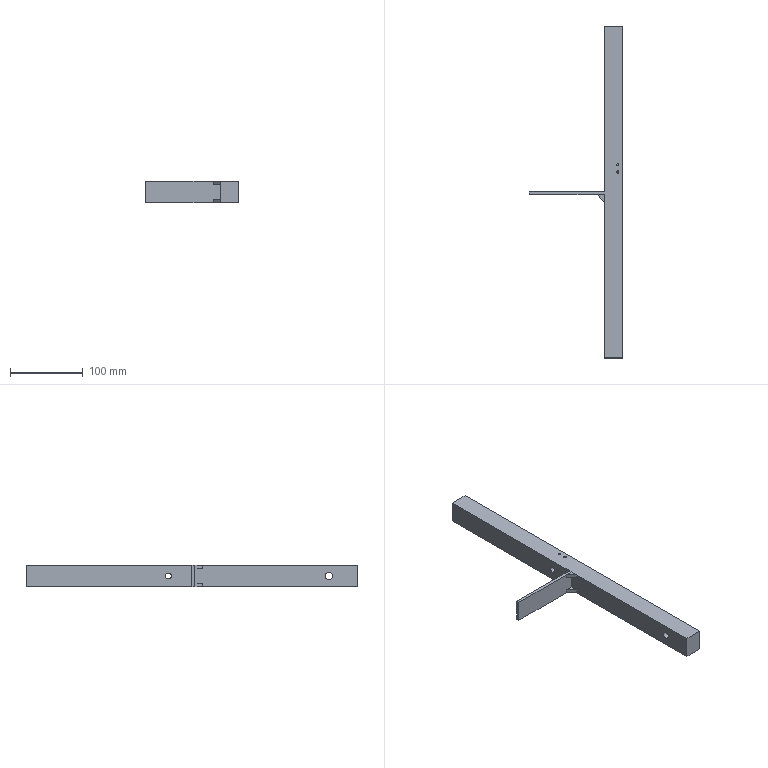Part | SolidWorks | features ICE 3, Cut 2, Gusset 2, Extrusion 1, Fillet 1, WeldmentFeature 1 | 3 solids | 37 faces | box 127.6 x 455 x 30 mm | volume 350644 mm3 | plane 24 | cylinder 13 | commonest cylinder face diameters 2 x5 3 x4 8 x2 10 x2
STEP:
#1=CARTESIAN_POINT('',(17.1,201.033,5.));
#2=VERTEX_POINT('',#1);
#3=CARTESIAN_POINT('',(20.1,201.033,5.));
#4=VERTEX_POINT('',#3);
#5=CARTESIAN_POINT('',(18.6,201.033,5.));
#6=DIRECTION('',(0.,0.,1.));
#7=DIRECTION('',(1.,0.,0.));
#8=AXIS2_PLACEMENT_3D('',#5,#6,#7);
#9=CIRCLE('',#8,1.5);
#10=EDGE_CURVE('',#2,#4,#9,.T.);
#11=ORIENTED_EDGE('',*,*,#10,.F.);
#12=CARTESIAN_POINT('',(17.1,201.033,15.));
#13=VERTEX_POINT('',#12);
#14=CARTESIAN_POINT('',(17.1,201.033,5.));
#15=DIRECTION('',(0.,0.,1.));
#16=VECTOR('',#15,1000.);
#17=LINE('',#14,#16);
#18=EDGE_CURVE('',#2,#13,#17,.T.);
#19=ORIENTED_EDGE('',*,*,#18,.T.);
#20=CARTESIAN_POINT('',(20.1,201.033,15.));
#21=VERTEX_POINT('',#20);
#22=CARTESIAN_POINT('',(18.6,201.033,15.));
#23=DIRECTION('',(0.,0.,1.));
#24=DIRECTION('',(1.,0.,0.));
#25=AXIS2_PLACEMENT_3D('',#22,#23,#24);
#26=CIRCLE('',#25,1.5);
#27=EDGE_CURVE('',#13,#21,#26,.T.);
#28=ORIENTED_EDGE('',*,*,#27,.T.);
#29=CARTESIAN_POINT('',(20.1,201.033,5.));
#30=DIRECTION('',(0.,0.,1.));
#31=VECTOR('',#30,1000.);
#32=LINE('',#29,#31);
#33=EDGE_CURVE('',#4,#21,#32,.T.);
#34=ORIENTED_EDGE('',*,*,#33,.F.);
#35=EDGE_LOOP('',(#11,#19,#28,#34));
#36=FACE_OUTER_BOUND('',#35,.T.);
#37=CARTESIAN_POINT('',(18.6,201.033,5.));
#38=DIRECTION('',(0.,0.,1.));
#39=DIRECTION('',(1.,0.,0.));
#40=AXIS2_PLACEMENT_3D('',#37,#38,#39);
#41=CYLINDRICAL_SURFACE('',#40,1.5);
#42=ADVANCED_FACE('',(#36),#41,.F.);
#43=CARTESIAN_POINT('',(17.1,211.033,5.));
#44=VERTEX_POINT('',#43);
#45=CARTESIAN_POINT('',(20.1,211.033,5.));
#46=VERTEX_POINT('',#45);
#47=CARTESIAN_POINT('',(18.6,211.033,5.));
#48=DIRECTION('',(0.,0.,1.));
#49=DIRECTION('',(1.,0.,0.));
#50=AXIS2_PLACEMENT_3D('',#47,#48,#49);
#51=CIRCLE('',#50,1.5);
#52=EDGE_CURVE('',#44,#46,#51,.T.);
#53=ORIENTED_EDGE('',*,*,#52,.F.);
#54=CARTESIAN_POINT('',(17.1,211.033,15.));
#55=VERTEX_POINT('',#54);
#56=CARTESIAN_POINT('',(17.1,211.033,5.));
#57=DIRECTION('',(0.,0.,1.));
#58=VECTOR('',#57,1000.);
#59=LINE('',#56,#58);
#60=EDGE_CURVE('',#44,#55,#59,.T.);
#61=ORIENTED_EDGE('',*,*,#60,.T.);
#62=CARTESIAN_POINT('',(20.1,211.033,15.));
#63=VERTEX_POINT('',#62);
#64=CARTESIAN_POINT('',(18.6,211.033,15.));
#65=DIRECTION('',(0.,0.,1.));
#66=DIRECTION('',(1.,0.,0.));
#67=AXIS2_PLACEMENT_3D('',#64,#65,#66);
#68=CIRCLE('',#67,1.5);
#69=EDGE_CURVE('',#55,#63,#68,.T.);
#70=ORIENTED_EDGE('',*,*,#69,.T.);
#71=CARTESIAN_POINT('',(20.1,211.033,5.));
#72=DIRECTION('',(0.,0.,1.));
#73=VECTOR('',#72,1000.);
#74=LINE('',#71,#73);
#75=EDGE_CURVE('',#46,#63,#74,.T.);
#76=ORIENTED_EDGE('',*,*,#75,.F.);
#77=EDGE_LOOP('',(#53,#61,#70,#76));
#78=FACE_OUTER_BOUND('',#77,.T.);
#79=CARTESIAN_POINT('',(18.6,211.033,5.));
#80=DIRECTION('',(0.,0.,1.));
#81=DIRECTION('',(1.,0.,0.));
#82=AXIS2_PLACEMENT_3D('',#79,#80,#81);
#83=CYLINDRICAL_SURFACE('',#82,1.5);
#84=ADVANCED_FACE('',(#78),#83,.F.);
#85=CARTESIAN_POINT('',(19.6,201.033,-5.));
#86=VERTEX_POINT('',#85);
#87=CARTESIAN_POINT('',(17.6,201.033,-5.));
#88=VERTEX_POINT('',#87);
#89=CARTESIAN_POINT('',(18.6,201.033,-5.));
#90=DIRECTION('',(0.,0.,-1.));
#91=DIRECTION('',(-1.,0.,0.));
#92=AXIS2_PLACEMENT_3D('',#89,#90,#91);
#93=CIRCLE('',#92,1.);
#94=EDGE_CURVE('',#86,#88,#93,.T.);
#95=ORIENTED_EDGE('',*,*,#94,.F.);
#96=CARTESIAN_POINT('',(19.6,201.033,-15.));
#97=VERTEX_POINT('',#96);
#98=CARTESIAN_POINT('',(19.6,201.033,-5.));
#99=DIRECTION('',(0.,0.,-1.));
#100=VECTOR('',#99,1000.);
#101=LINE('',#98,#100);
#102=EDGE_CURVE('',#86,#97,#101,.T.);
#103=ORIENTED_EDGE('',*,*,#102,.T.);
#104=CARTESIAN_POINT('',(17.6,201.033,-15.));
#105=VERTEX_POINT('',#104);
#106=CARTESIAN_POINT('',(18.6,201.033,-15.));
#107=DIRECTION('',(0.,0.,-1.));
#108=DIRECTION('',(-1.,0.,0.));
#109=AXIS2_PLACEMENT_3D('',#106,#107,#108);
#110=CIRCLE('',#109,1.);
#111=EDGE_CURVE('',#97,#105,#110,.T.);
#112=ORIENTED_EDGE('',*,*,#111,.T.);
#113=CARTESIAN_POINT('',(17.6,201.033,-5.));
#114=DIRECTION('',(0.,0.,-1.));
#115=VECTOR('',#114,1000.);
#116=LINE('',#113,#115);
#117=EDGE_CURVE('',#88,#105,#116,.T.);
#118=ORIENTED_EDGE('',*,*,#117,.F.);
#119=EDGE_LOOP('',(#95,#103,#112,#118));
#120=FACE_OUTER_BOUND('',#119,.T.);
#121=CARTESIAN_POINT('',(18.6,201.033,-5.));
#122=DIRECTION('',(0.,0.,-1.));
#123=DIRECTION('',(-1.,0.,0.));
#124=AXIS2_PLACEMENT_3D('',#121,#122,#123);
#125=CYLINDRICAL_SURFACE('',#124,1.);
#126=ADVANCED_FACE('',(#120),#125,.F.);
#127=CARTESIAN_POINT('',(19.6,211.033,-5.));
#128=VERTEX_POINT('',#127);
#129=CARTESIAN_POINT('',(17.6,211.033,-5.));
#130=VERTEX_POINT('',#129);
#131=CARTESIAN_POINT('',(18.6,211.033,-5.));
#132=DIRECTION('',(0.,0.,-1.));
#133=DIRECTION('',(-1.,0.,0.));
#134=AXIS2_PLACEMENT_3D('',#131,#132,#133);
#135=CIRCLE('',#134,1.);
#136=EDGE_CURVE('',#128,#130,#135,.T.);
#137=ORIENTED_EDGE('',*,*,#136,.F.);
#138=CARTESIAN_POINT('',(19.6,211.033,-15.));
#139=VERTEX_POINT('',#138);
#140=CARTESIAN_POINT('',(19.6,211.033,-5.));
#141=DIRECTION('',(0.,0.,-1.));
#142=VECTOR('',#141,1000.);
#143=LINE('',#140,#142);
#144=EDGE_CURVE('',#128,#139,#143,.T.);
#145=ORIENTED_EDGE('',*,*,#144,.T.);
#146=CARTESIAN_POINT('',(17.6,211.033,-15.));
#147=VERTEX_POINT('',#146);
#148=CARTESIAN_POINT('',(18.6,211.033,-15.));
#149=DIRECTION('',(0.,0.,-1.));
#150=DIRECTION('',(-1.,0.,0.));
#151=AXIS2_PLACEMENT_3D('',#148,#149,#150);
#152=CIRCLE('',#151,1.);
#153=EDGE_CURVE('',#139,#147,#152,.T.);
#154=ORIENTED_EDGE('',*,*,#153,.T.);
#155=CARTESIAN_POINT('',(17.6,211.033,-5.));
#156=DIRECTION('',(0.,0.,-1.));
#157=VECTOR('',#156,1000.);
#158=LINE('',#155,#157);
#159=EDGE_CURVE('',#130,#147,#158,.T.);
#160=ORIENTED_EDGE('',*,*,#159,.F.);
#161=EDGE_LOOP('',(#137,#145,#154,#160));
#162=FACE_OUTER_BOUND('',#161,.T.);
#163=CARTESIAN_POINT('',(18.6,211.033,-5.));
#164=DIRECTION('',(0.,0.,-1.));
#165=DIRECTION('',(-1.,0.,0.));
#166=AXIS2_PLACEMENT_3D('',#163,#164,#165);
#167=CYLINDRICAL_SURFACE('',#166,1.);
#168=ADVANCED_FACE('',(#162),#167,.F.);
#169=CARTESIAN_POINT('',(25.,-13.967,-5.));
#170=VERTEX_POINT('',#169);
#171=CARTESIAN_POINT('',(25.,-13.967,5.));
#172=VERTEX_POINT('',#171);
#173=CARTESIAN_POINT('',(25.,-13.967,0.));
#174=DIRECTION('',(-1.,0.,0.));
#175=DIRECTION('',(0.,-1.,0.));
#176=AXIS2_PLACEMENT_3D('',#173,#174,#175);
#177=CIRCLE('',#176,5.);
#178=EDGE_CURVE('',#170,#172,#177,.T.);
#179=ORIENTED_EDGE('',*,*,#178,.F.);
#180=CARTESIAN_POINT('',(0.,-13.967,-5.));
#181=VERTEX_POINT('',#180);
#182=CARTESIAN_POINT('',(66.,-13.967,-5.));
#183=DIRECTION('',(-1.,0.,0.));
#184=VECTOR('',#183,1000.);
#185=LINE('',#182,#184);
#186=EDGE_CURVE('',#170,#181,#185,.T.);
#187=ORIENTED_EDGE('',*,*,#186,.T.);
#188=CARTESIAN_POINT('',(0.,-13.967,5.));
#189=VERTEX_POINT('',#188);
#190=CARTESIAN_POINT('',(0.,-13.967,0.));
#191=DIRECTION('',(1.,0.,0.));
#192=DIRECTION('',(0.,0.,-1.));
#193=AXIS2_PLACEMENT_3D('',#190,#191,#192);
#194=CIRCLE('',#193,5.);
#195=EDGE_CURVE('',#189,#181,#194,.T.);
#196=ORIENTED_EDGE('',*,*,#195,.F.);
#197=CARTESIAN_POINT('',(66.,-13.967,5.));
#198=DIRECTION('',(-1.,0.,0.));
#199=VECTOR('',#198,1000.);
#200=LINE('',#197,#199);
#201=EDGE_CURVE('',#172,#189,#200,.T.);
#202=ORIENTED_EDGE('',*,*,#201,.F.);
#203=EDGE_LOOP('',(#179,#187,#196,#202));
#204=FACE_OUTER_BOUND('',#203,.T.);
#205=CARTESIAN_POINT('',(66.,-13.967,0.));
#206=DIRECTION('',(-1.,0.,0.));
#207=DIRECTION('',(0.,0.,1.));
#208=AXIS2_PLACEMENT_3D('',#205,#206,#207);
#209=CYLINDRICAL_SURFACE('',#208,5.);
#210=ADVANCED_FACE('',(#204),#209,.F.);
#211=CARTESIAN_POINT('',(25.,206.033,-4.));
#212=VERTEX_POINT('',#211);
#213=CARTESIAN_POINT('',(25.,206.033,4.));
#214=VERTEX_POINT('',#213);
#215=CARTESIAN_POINT('',(25.,206.033,0.));
#216=DIRECTION('',(-1.,0.,0.));
#217=DIRECTION('',(0.,-1.,0.));
#218=AXIS2_PLACEMENT_3D('',#215,#216,#217);
#219=CIRCLE('',#218,4.);
#220=EDGE_CURVE('',#212,#214,#219,.T.);
#221=ORIENTED_EDGE('',*,*,#220,.F.);
#222=CARTESIAN_POINT('',(0.,206.033,-4.));
#223=VERTEX_POINT('',#222);
#224=CARTESIAN_POINT('',(66.,206.033,-4.));
#225=DIRECTION('',(-1.,0.,0.));
#226=VECTOR('',#225,1000.);
#227=LINE('',#224,#226);
#228=EDGE_CURVE('',#212,#223,#227,.T.);
#229=ORIENTED_EDGE('',*,*,#228,.T.);
#230=CARTESIAN_POINT('',(0.,206.033,4.));
#231=VERTEX_POINT('',#230);
#232=CARTESIAN_POINT('',(0.,206.033,0.));
#233=DIRECTION('',(1.,0.,0.));
#234=DIRECTION('',(0.,0.,-1.));
#235=AXIS2_PLACEMENT_3D('',#232,#233,#234);
#236=CIRCLE('',#235,4.);
#237=EDGE_CURVE('',#231,#223,#236,.T.);
#238=ORIENTED_EDGE('',*,*,#237,.F.);
#239=CARTESIAN_POINT('',(66.,206.033,4.));
#240=DIRECTION('',(-1.,0.,0.));
#241=VECTOR('',#240,1000.);
#242=LINE('',#239,#241);
#243=EDGE_CURVE('',#214,#231,#242,.T.);
#244=ORIENTED_EDGE('',*,*,#243,.F.);
#245=EDGE_LOOP('',(#221,#229,#238,#244));
#246=FACE_OUTER_BOUND('',#245,.T.);
#247=CARTESIAN_POINT('',(66.,206.033,0.));
#248=DIRECTION('',(-1.,0.,0.));
#249=DIRECTION('',(0.,0.,1.));
#250=AXIS2_PLACEMENT_3D('',#247,#248,#249);
#251=CYLINDRICAL_SURFACE('',#250,4.);
#252=ADVANCED_FACE('',(#246),#251,.F.);
#253=ORIENTED_EDGE('',*,*,#237,.T.);
#254=CARTESIAN_POINT('',(0.,206.033,0.));
#255=DIRECTION('',(1.,0.,0.));
#256=DIRECTION('',(0.,0.,-1.));
#257=AXIS2_PLACEMENT_3D('',#254,#255,#256);
#258=CIRCLE('',#257,4.);
#259=EDGE_CURVE('',#223,#231,#258,.T.);
#260=ORIENTED_EDGE('',*,*,#259,.T.);
#261=EDGE_LOOP('',(#253,#260));
#262=FACE_BOUND('',#261,.T.);
#263=CARTESIAN_POINT('',(0.,401.033,-15.));
#264=VERTEX_POINT('',#263);
#265=CARTESIAN_POINT('',(0.,174.533,-15.));
#266=VERTEX_POINT('',#265);
#267=CARTESIAN_POINT('',(0.,0.,-15.));
#268=DIRECTION('',(0.,-1.,0.));
#269=VECTOR('',#268,1000.);
#270=LINE('',#267,#269);
#271=EDGE_CURVE('',#264,#266,#270,.T.);
#272=ORIENTED_EDGE('',*,*,#271,.T.);
#273=CARTESIAN_POINT('',(0.,174.533,15.));
#274=VERTEX_POINT('',#273);
#275=CARTESIAN_POINT('',(0.,174.533,15.));
#276=DIRECTION('',(0.,0.,1.));
#277=VECTOR('',#276,1000.);
#278=LINE('',#275,#277);
#279=EDGE_CURVE('',#266,#274,#278,.T.);
#280=ORIENTED_EDGE('',*,*,#279,.T.);
#281=CARTESIAN_POINT('',(0.,401.033,15.));
#282=VERTEX_POINT('',#281);
#283=CARTESIAN_POINT('',(0.,-53.967,15.));
#284=DIRECTION('',(0.,-1.,0.));
#285=VECTOR('',#284,1000.);
#286=LINE('',#283,#285);
#287=EDGE_CURVE('',#282,#274,#286,.T.);
#288=ORIENTED_EDGE('',*,*,#287,.F.);
#289=CARTESIAN_POINT('',(0.,401.033,-15.));
#290=DIRECTION('',(0.,0.,1.));
#291=VECTOR('',#290,1000.);
#292=LINE('',#289,#291);
#293=EDGE_CURVE('',#264,#282,#292,.T.);
#294=ORIENTED_EDGE('',*,*,#293,.F.);
#295=EDGE_LOOP('',(#272,#280,#288,#294));
#296=FACE_OUTER_BOUND('',#295,.T.);
#297=CARTESIAN_POINT('',(0.,0.,15.));
#298=DIRECTION('',(1.,0.,0.));
#299=DIRECTION('',(0.,0.,-1.));
#300=AXIS2_PLACEMENT_3D('',#297,#298,#299);
#301=PLANE('',#300);
#302=ADVANCED_FACE('',(#262,#296),#301,.F.);
#303=CARTESIAN_POINT('',(0.,-53.967,-15.));
#304=VERTEX_POINT('',#303);
#305=CARTESIAN_POINT('',(25.,-53.967,-15.));
#306=VERTEX_POINT('',#305);
#307=CARTESIAN_POINT('',(25.,-53.967,-15.));
#308=DIRECTION('',(1.,0.,0.));
#309=VECTOR('',#308,1000.);
#310=LINE('',#307,#309);
#311=EDGE_CURVE('',#304,#306,#310,.T.);
#312=ORIENTED_EDGE('',*,*,#311,.T.);
#313=CARTESIAN_POINT('',(25.,-53.967,15.));
#314=VERTEX_POINT('',#313);
#315=CARTESIAN_POINT('',(25.,-53.967,15.));
#316=DIRECTION('',(0.,0.,-1.));
#317=VECTOR('',#316,1000.);
#318=LINE('',#315,#317);
#319=EDGE_CURVE('',#314,#306,#318,.T.);
#320=ORIENTED_EDGE('',*,*,#319,.F.);
#321=CARTESIAN_POINT('',(0.,-53.967,15.));
#322=VERTEX_POINT('',#321);
#323=CARTESIAN_POINT('',(25.,-53.967,15.));
#324=DIRECTION('',(1.,0.,0.));
#325=VECTOR('',#324,1000.);
#326=LINE('',#323,#325);
#327=EDGE_CURVE('',#322,#314,#326,.T.);
#328=ORIENTED_EDGE('',*,*,#327,.F.);
#329=CARTESIAN_POINT('',(0.,-53.967,15.));
#330=DIRECTION('',(0.,0.,-1.));
#331=VECTOR('',#330,1000.);
#332=LINE('',#329,#331);
#333=EDGE_CURVE('',#322,#304,#332,.T.);
#334=ORIENTED_EDGE('',*,*,#333,.T.);
#335=EDGE_LOOP('',(#312,#320,#328,#334));
#336=FACE_OUTER_BOUND('',#335,.T.);
#337=CARTESIAN_POINT('',(25.,-53.967,15.));
#338=DIRECTION('',(0.,1.,0.));
#339=DIRECTION('',(-1.,0.,0.));
#340=AXIS2_PLACEMENT_3D('',#337,#338,#339);
#341=PLANE('',#340);
#342=ADVANCED_FACE('',(#336),#341,.F.);
#343=CARTESIAN_POINT('',(25.,-13.967,0.));
#344=DIRECTION('',(-1.,0.,0.));
#345=DIRECTION('',(0.,-1.,0.));
#346=AXIS2_PLACEMENT_3D('',#343,#344,#345);
#347=CIRCLE('',#346,5.);
#348=EDGE_CURVE('',#172,#170,#347,.T.);
#349=ORIENTED_EDGE('',*,*,#348,.T.);
#350=ORIENTED_EDGE('',*,*,#178,.T.);
#351=EDGE_LOOP('',(#349,#350));
#352=FACE_BOUND('',#351,.T.);
#353=CARTESIAN_POINT('',(25.,206.033,0.));
#354=DIRECTION('',(-1.,0.,0.));
#355=DIRECTION('',(0.,-1.,0.));
#356=AXIS2_PLACEMENT_3D('',#353,#354,#355);
#357=CIRCLE('',#356,4.);
#358=EDGE_CURVE('',#214,#212,#357,.T.);
#359=ORIENTED_EDGE('',*,*,#358,.T.);
#360=ORIENTED_EDGE('',*,*,#220,.T.);
#361=EDGE_LOOP('',(#359,#360));
#362=FACE_BOUND('',#361,.T.);
#363=CARTESIAN_POINT('',(25.,401.033,-15.));
#364=VERTEX_POINT('',#363);
#365=CARTESIAN_POINT('',(25.,246.033,-15.));
#366=DIRECTION('',(0.,1.,0.));
#367=VECTOR('',#366,1000.);
#368=LINE('',#365,#367);
#369=EDGE_CURVE('',#306,#364,#368,.T.);
#370=ORIENTED_EDGE('',*,*,#369,.T.);
#371=CARTESIAN_POINT('',(25.,401.033,15.));
#372=VERTEX_POINT('',#371);
#373=CARTESIAN_POINT('',(25.,401.033,15.));
#374=DIRECTION('',(0.,0.,-1.));
#375=VECTOR('',#374,1000.);
#376=LINE('',#373,#375);
#377=EDGE_CURVE('',#372,#364,#376,.T.);
#378=ORIENTED_EDGE('',*,*,#377,.F.);
#379=CARTESIAN_POINT('',(25.,-38.967,15.));
#380=DIRECTION('',(0.,1.,0.));
#381=VECTOR('',#380,1000.);
#382=LINE('',#379,#381);
#383=EDGE_CURVE('',#314,#372,#382,.T.);
#384=ORIENTED_EDGE('',*,*,#383,.F.);
#385=ORIENTED_EDGE('',*,*,#319,.T.);
#386=EDGE_LOOP('',(#370,#378,#384,#385));
#387=FACE_OUTER_BOUND('',#386,.T.);
#388=CARTESIAN_POINT('',(25.,246.033,15.));
#389=DIRECTION('',(-1.,0.,0.));
#390=DIRECTION('',(0.,-1.,0.));
#391=AXIS2_PLACEMENT_3D('',#388,#389,#390);
#392=PLANE('',#391);
#393=ADVANCED_FACE('',(#352,#362,#387),#392,.F.);
#394=ORIENTED_EDGE('',*,*,#195,.T.);
#395=CARTESIAN_POINT('',(0.,-13.967,0.));
#396=DIRECTION('',(1.,0.,0.));
#397=DIRECTION('',(0.,0.,-1.));
#398=AXIS2_PLACEMENT_3D('',#395,#396,#397);
#399=CIRCLE('',#398,5.);
#400=EDGE_CURVE('',#181,#189,#399,.T.);
#401=ORIENTED_EDGE('',*,*,#400,.T.);
#402=EDGE_LOOP('',(#394,#401));
#403=FACE_BOUND('',#402,.T.);
#404=CARTESIAN_POINT('',(0.,169.533,15.));
#405=VERTEX_POINT('',#404);
#406=CARTESIAN_POINT('',(0.,-53.967,15.));
#407=DIRECTION('',(0.,-1.,0.));
#408=VECTOR('',#407,1000.);
#409=LINE('',#406,#408);
#410=EDGE_CURVE('',#405,#322,#409,.T.);
#411=ORIENTED_EDGE('',*,*,#410,.F.);
#412=CARTESIAN_POINT('',(0.,169.533,-15.));
#413=VERTEX_POINT('',#412);
#414=CARTESIAN_POINT('',(0.,169.533,117.678));
#415=DIRECTION('',(0.,0.,-1.));
#416=VECTOR('',#415,1000.);
#417=LINE('',#414,#416);
#418=EDGE_CURVE('',#405,#413,#417,.T.);
#419=ORIENTED_EDGE('',*,*,#418,.T.);
#420=CARTESIAN_POINT('',(0.,0.,-15.));
#421=DIRECTION('',(0.,-1.,0.));
#422=VECTOR('',#421,1000.);
#423=LINE('',#420,#422);
#424=EDGE_CURVE('',#413,#304,#423,.T.);
#425=ORIENTED_EDGE('',*,*,#424,.T.);
#426=ORIENTED_EDGE('',*,*,#333,.F.);
#427=EDGE_LOOP('',(#411,#419,#425,#426));
#428=FACE_OUTER_BOUND('',#427,.T.);
#429=CARTESIAN_POINT('',(0.,0.,15.));
#430=DIRECTION('',(1.,0.,0.));
#431=DIRECTION('',(0.,0.,-1.));
#432=AXIS2_PLACEMENT_3D('',#429,#430,#431);
#433=PLANE('',#432);
#434=ADVANCED_FACE('',(#403,#428),#433,.F.);
#435=CARTESIAN_POINT('',(18.6,201.033,15.));
#436=DIRECTION('',(0.,0.,1.));
#437=DIRECTION('',(1.,0.,0.));
#438=AXIS2_PLACEMENT_3D('',#435,#436,#437);
#439=CIRCLE('',#438,1.5);
#440=EDGE_CURVE('',#21,#13,#439,.T.);
#441=ORIENTED_EDGE('',*,*,#440,.F.);
#442=ORIENTED_EDGE('',*,*,#27,.F.);
#443=EDGE_LOOP('',(#441,#442));
#444=FACE_BOUND('',#443,.T.);
#445=CARTESIAN_POINT('',(18.6,211.033,15.));
#446=DIRECTION('',(0.,0.,1.));
#447=DIRECTION('',(1.,0.,0.));
#448=AXIS2_PLACEMENT_3D('',#445,#446,#447);
#449=CIRCLE('',#448,1.5);
#450=EDGE_CURVE('',#63,#55,#449,.T.);
#451=ORIENTED_EDGE('',*,*,#450,.F.);
#452=ORIENTED_EDGE('',*,*,#69,.F.);
#453=EDGE_LOOP('',(#451,#452));
#454=FACE_BOUND('',#453,.T.);
#455=ORIENTED_EDGE('',*,*,#287,.T.);
#456=CARTESIAN_POINT('',(-1.,173.533,15.));
#457=VERTEX_POINT('',#456);
#458=CARTESIAN_POINT('',(-1.,174.533,15.));
#459=DIRECTION('',(0.,0.,-1.));
#460=DIRECTION('',(-1.,0.,0.));
#461=AXIS2_PLACEMENT_3D('',#458,#459,#460);
#462=CIRCLE('',#461,1.);
#463=EDGE_CURVE('',#274,#457,#462,.T.);
#464=ORIENTED_EDGE('',*,*,#463,.T.);
#465=CARTESIAN_POINT('',(-102.6,173.533,15.));
#466=VERTEX_POINT('',#465);
#467=CARTESIAN_POINT('',(0.,173.533,15.));
#468=DIRECTION('',(-1.,0.,0.));
#469=VECTOR('',#468,1000.);
#470=LINE('',#467,#469);
#471=EDGE_CURVE('',#457,#466,#470,.T.);
#472=ORIENTED_EDGE('',*,*,#471,.T.);
#473=CARTESIAN_POINT('',(-102.6,169.533,15.));
#474=VERTEX_POINT('',#473);
#475=CARTESIAN_POINT('',(-102.6,173.533,15.));
#476=DIRECTION('',(0.,-1.,0.));
#477=VECTOR('',#476,1000.);
#478=LINE('',#475,#477);
#479=EDGE_CURVE('',#466,#474,#478,.T.);
#480=ORIENTED_EDGE('',*,*,#479,.T.);
#481=CARTESIAN_POINT('',(-102.6,169.533,15.));
#482=DIRECTION('',(1.,0.,0.));
#483=VECTOR('',#482,1000.);
#484=LINE('',#481,#483);
#485=EDGE_CURVE('',#474,#405,#484,.T.);
#486=ORIENTED_EDGE('',*,*,#485,.T.);
#487=ORIENTED_EDGE('',*,*,#410,.T.);
#488=ORIENTED_EDGE('',*,*,#327,.T.);
#489=ORIENTED_EDGE('',*,*,#383,.T.);
#490=CARTESIAN_POINT('',(0.,401.033,15.));
#491=DIRECTION('',(1.,0.,0.));
#492=VECTOR('',#491,1000.);
#493=LINE('',#490,#492);
#494=EDGE_CURVE('',#282,#372,#493,.T.);
#495=ORIENTED_EDGE('',*,*,#494,.F.);
#496=EDGE_LOOP('',(#455,#464,#472,#480,#486,#487,#488,#489,#495));
#497=FACE_OUTER_BOUND('',#496,.T.);
#498=CARTESIAN_POINT('',(0.,0.,15.));
#499=DIRECTION('',(0.,0.,-1.));
#500=DIRECTION('',(-1.,0.,0.));
#501=AXIS2_PLACEMENT_3D('',#498,#499,#500);
#502=PLANE('',#501);
#503=ADVANCED_FACE('',(#444,#454,#497),#502,.F.);
#504=CARTESIAN_POINT('',(18.6,201.033,-15.));
#505=DIRECTION('',(0.,0.,-1.));
#506=DIRECTION('',(-1.,0.,0.));
#507=AXIS2_PLACEMENT_3D('',#504,#505,#506);
#508=CIRCLE('',#507,1.);
#509=EDGE_CURVE('',#105,#97,#508,.T.);
#510=ORIENTED_EDGE('',*,*,#509,.F.);
#511=ORIENTED_EDGE('',*,*,#111,.F.);
#512=EDGE_LOOP('',(#510,#511));
#513=FACE_BOUND('',#512,.T.);
#514=CARTESIAN_POINT('',(18.6,211.033,-15.));
#515=DIRECTION('',(0.,0.,-1.));
#516=DIRECTION('',(-1.,0.,0.));
#517=AXIS2_PLACEMENT_3D('',#514,#515,#516);
#518=CIRCLE('',#517,1.);
#519=EDGE_CURVE('',#147,#139,#518,.T.);
#520=ORIENTED_EDGE('',*,*,#519,.F.);
#521=ORIENTED_EDGE('',*,*,#153,.F.);
#522=EDGE_LOOP('',(#520,#521));
#523=FACE_BOUND('',#522,.T.);
#524=ORIENTED_EDGE('',*,*,#311,.F.);
#525=ORIENTED_EDGE('',*,*,#424,.F.);
#526=CARTESIAN_POINT('',(-102.6,169.533,-15.));
#527=VERTEX_POINT('',#526);
#528=CARTESIAN_POINT('',(-102.6,169.533,-15.));
#529=DIRECTION('',(-1.,0.,0.));
#530=VECTOR('',#529,1000.);
#531=LINE('',#528,#530);
#532=EDGE_CURVE('',#413,#527,#531,.T.);
#533=ORIENTED_EDGE('',*,*,#532,.T.);
#534=CARTESIAN_POINT('',(-102.6,173.533,-15.));
#535=VERTEX_POINT('',#534);
#536=CARTESIAN_POINT('',(-102.6,173.533,-15.));
#537=DIRECTION('',(0.,1.,0.));
#538=VECTOR('',#537,1000.);
#539=LINE('',#536,#538);
#540=EDGE_CURVE('',#527,#535,#539,.T.);
#541=ORIENTED_EDGE('',*,*,#540,.T.);
#542=CARTESIAN_POINT('',(-1.,173.533,-15.));
#543=VERTEX_POINT('',#542);
#544=CARTESIAN_POINT('',(0.,173.533,-15.));
#545=DIRECTION('',(1.,0.,0.));
#546=VECTOR('',#545,1000.);
#547=LINE('',#544,#546);
#548=EDGE_CURVE('',#535,#543,#547,.T.);
#549=ORIENTED_EDGE('',*,*,#548,.T.);
#550=CARTESIAN_POINT('',(-1.,174.533,-15.));
#551=DIRECTION('',(0.,0.,1.));
#552=DIRECTION('',(-1.,0.,0.));
#553=AXIS2_PLACEMENT_3D('',#550,#551,#552);
#554=CIRCLE('',#553,1.);
#555=EDGE_CURVE('',#543,#266,#554,.T.);
#556=ORIENTED_EDGE('',*,*,#555,.T.);
#557=ORIENTED_EDGE('',*,*,#271,.F.);
#558=CARTESIAN_POINT('',(25.,401.033,-15.));
#559=DIRECTION('',(-1.,0.,0.));
#560=VECTOR('',#559,1000.);
#561=LINE('',#558,#560);
#562=EDGE_CURVE('',#364,#264,#561,.T.);
#563=ORIENTED_EDGE('',*,*,#562,.F.);
#564=ORIENTED_EDGE('',*,*,#369,.F.);
#565=EDGE_LOOP('',(#524,#525,#533,#541,#549,#556,#557,#563,#564));
#566=FACE_OUTER_BOUND('',#565,.T.);
#567=CARTESIAN_POINT('',(0.,0.,-15.));
#568=DIRECTION('',(0.,0.,-1.));
#569=DIRECTION('',(-1.,0.,0.));
#570=AXIS2_PLACEMENT_3D('',#567,#568,#569);
#571=PLANE('',#570);
#572=ADVANCED_FACE('',(#513,#523,#566),#571,.T.);
#573=ORIENTED_EDGE('',*,*,#228,.F.);
#574=ORIENTED_EDGE('',*,*,#358,.F.);
#575=ORIENTED_EDGE('',*,*,#243,.T.);
#576=ORIENTED_EDGE('',*,*,#259,.F.);
#577=EDGE_LOOP('',(#573,#574,#575,#576));
#578=FACE_OUTER_BOUND('',#577,.T.);
#579=CARTESIAN_POINT('',(66.,206.033,0.));
#580=DIRECTION('',(-1.,0.,0.));
#581=DIRECTION('',(0.,0.,1.));
#582=AXIS2_PLACEMENT_3D('',#579,#580,#581);
#583=CYLINDRICAL_SURFACE('',#582,4.);
#584=ADVANCED_FACE('',(#578),#583,.F.);
#585=ORIENTED_EDGE('',*,*,#186,.F.);
#586=ORIENTED_EDGE('',*,*,#348,.F.);
#587=ORIENTED_EDGE('',*,*,#201,.T.);
#588=ORIENTED_EDGE('',*,*,#400,.F.);
#589=EDGE_LOOP('',(#585,#586,#587,#588));
#590=FACE_OUTER_BOUND('',#589,.T.);
#591=CARTESIAN_POINT('',(66.,-13.967,0.));
#592=DIRECTION('',(-1.,0.,0.));
#593=DIRECTION('',(0.,0.,1.));
#594=AXIS2_PLACEMENT_3D('',#591,#592,#593);
#595=CYLINDRICAL_SURFACE('',#594,5.);
#596=ADVANCED_FACE('',(#590),#595,.F.);
#597=ORIENTED_EDGE('',*,*,#471,.F.);
#598=CARTESIAN_POINT('',(-1.,173.533,117.678));
#599=DIRECTION('',(0.,0.,-1.));
#600=VECTOR('',#599,1000.);
#601=LINE('',#598,#600);
#602=EDGE_CURVE('',#457,#543,#601,.T.);
#603=ORIENTED_EDGE('',*,*,#602,.T.);
#604=ORIENTED_EDGE('',*,*,#548,.F.);
#605=CARTESIAN_POINT('',(-102.6,173.533,117.678));
#606=DIRECTION('',(0.,0.,-1.));
#607=VECTOR('',#606,1000.);
#608=LINE('',#605,#607);
#609=EDGE_CURVE('',#466,#535,#608,.T.);
#610=ORIENTED_EDGE('',*,*,#609,.F.);
#611=EDGE_LOOP('',(#597,#603,#604,#610));
#612=FACE_OUTER_BOUND('',#611,.T.);
#613=CARTESIAN_POINT('',(0.,173.533,117.678));
#614=DIRECTION('',(0.,1.,0.));
#615=DIRECTION('',(0.,0.,1.));
#616=AXIS2_PLACEMENT_3D('',#613,#614,#615);
#617=PLANE('',#616);
#618=ADVANCED_FACE('',(#612),#617,.T.);
#619=ORIENTED_EDGE('',*,*,#479,.F.);
#620=ORIENTED_EDGE('',*,*,#609,.T.);
#621=ORIENTED_EDGE('',*,*,#540,.F.);
#622=CARTESIAN_POINT('',(-102.6,169.533,117.678));
#623=DIRECTION('',(0.,0.,-1.));
#624=VECTOR('',#623,1000.);
#625=LINE('',#622,#624);
#626=EDGE_CURVE('',#474,#527,#625,.T.);
#627=ORIENTED_EDGE('',*,*,#626,.F.);
#628=EDGE_LOOP('',(#619,#620,#621,#627));
#629=FACE_OUTER_BOUND('',#628,.T.);
#630=CARTESIAN_POINT('',(-102.6,173.533,117.678));
#631=DIRECTION('',(-1.,0.,0.));
#632=DIRECTION('',(0.,0.,1.));
#633=AXIS2_PLACEMENT_3D('',#630,#631,#632);
#634=PLANE('',#633);
#635=ADVANCED_FACE('',(#629),#634,.T.);
#636=ORIENTED_EDGE('',*,*,#485,.F.);
#637=ORIENTED_EDGE('',*,*,#626,.T.);
#638=ORIENTED_EDGE('',*,*,#532,.F.);
#639=ORIENTED_EDGE('',*,*,#418,.F.);
#640=EDGE_LOOP('',(#636,#637,#638,#639));
#641=FACE_OUTER_BOUND('',#640,.T.);
#642=CARTESIAN_POINT('',(-102.6,169.533,117.678));
#643=DIRECTION('',(0.,-1.,0.));
#644=DIRECTION('',(1.,0.,0.));
#645=AXIS2_PLACEMENT_3D('',#642,#643,#644);
#646=PLANE('',#645);
#647=ADVANCED_FACE('',(#641),#646,.T.);
#648=ORIENTED_EDGE('',*,*,#377,.T.);
#649=ORIENTED_EDGE('',*,*,#562,.T.);
#650=ORIENTED_EDGE('',*,*,#293,.T.);
#651=ORIENTED_EDGE('',*,*,#494,.T.);
#652=EDGE_LOOP('',(#648,#649,#650,#651));
#653=FACE_OUTER_BOUND('',#652,.T.);
#654=CARTESIAN_POINT('',(0.,401.033,0.));
#655=DIRECTION('',(0.,1.,0.));
#656=DIRECTION('',(0.,0.,1.));
#657=AXIS2_PLACEMENT_3D('',#654,#655,#656);
#658=PLANE('',#657);
#659=ADVANCED_FACE('',(#653),#658,.T.);
#660=ORIENTED_EDGE('',*,*,#144,.F.);
#661=CARTESIAN_POINT('',(18.6,211.033,-5.));
#662=DIRECTION('',(0.,0.,-1.));
#663=DIRECTION('',(-1.,0.,0.));
#664=AXIS2_PLACEMENT_3D('',#661,#662,#663);
#665=CIRCLE('',#664,1.);
#666=EDGE_CURVE('',#130,#128,#665,.T.);
#667=ORIENTED_EDGE('',*,*,#666,.F.);
#668=ORIENTED_EDGE('',*,*,#159,.T.);
#669=ORIENTED_EDGE('',*,*,#519,.T.);
#670=EDGE_LOOP('',(#660,#667,#668,#669));
#671=FACE_OUTER_BOUND('',#670,.T.);
#672=CARTESIAN_POINT('',(18.6,211.033,-5.));
#673=DIRECTION('',(0.,0.,-1.));
#674=DIRECTION('',(-1.,0.,0.));
#675=AXIS2_PLACEMENT_3D('',#672,#673,#674);
#676=CYLINDRICAL_SURFACE('',#675,1.);
#677=ADVANCED_FACE('',(#671),#676,.F.);
#678=ORIENTED_EDGE('',*,*,#666,.T.);
#679=ORIENTED_EDGE('',*,*,#136,.T.);
#680=EDGE_LOOP('',(#678,#679));
#681=FACE_OUTER_BOUND('',#680,.T.);
#682=CARTESIAN_POINT('',(18.6,211.033,-5.));
#683=DIRECTION('',(0.,0.,-1.));
#684=DIRECTION('',(-1.,0.,0.));
#685=AXIS2_PLACEMENT_3D('',#682,#683,#684);
#686=PLANE('',#685);
#687=ADVANCED_FACE('',(#681),#686,.T.);
#688=ORIENTED_EDGE('',*,*,#102,.F.);
#689=CARTESIAN_POINT('',(18.6,201.033,-5.));
#690=DIRECTION('',(0.,0.,-1.));
#691=DIRECTION('',(-1.,0.,0.));
#692=AXIS2_PLACEMENT_3D('',#689,#690,#691);
#693=CIRCLE('',#692,1.);
#694=EDGE_CURVE('',#88,#86,#693,.T.);
#695=ORIENTED_EDGE('',*,*,#694,.F.);
#696=ORIENTED_EDGE('',*,*,#117,.T.);
#697=ORIENTED_EDGE('',*,*,#509,.T.);
#698=EDGE_LOOP('',(#688,#695,#696,#697));
#699=FACE_OUTER_BOUND('',#698,.T.);
#700=CARTESIAN_POINT('',(18.6,201.033,-5.));
#701=DIRECTION('',(0.,0.,-1.));
#702=DIRECTION('',(-1.,0.,0.));
#703=AXIS2_PLACEMENT_3D('',#700,#701,#702);
#704=CYLINDRICAL_SURFACE('',#703,1.);
#705=ADVANCED_FACE('',(#699),#704,.F.);
#706=ORIENTED_EDGE('',*,*,#694,.T.);
#707=ORIENTED_EDGE('',*,*,#94,.T.);
#708=EDGE_LOOP('',(#706,#707));
#709=FACE_OUTER_BOUND('',#708,.T.);
#710=CARTESIAN_POINT('',(18.6,201.033,-5.));
#711=DIRECTION('',(0.,0.,-1.));
#712=DIRECTION('',(-1.,0.,0.));
#713=AXIS2_PLACEMENT_3D('',#710,#711,#712);
#714=PLANE('',#713);
#715=ADVANCED_FACE('',(#709),#714,.T.);
#716=ORIENTED_EDGE('',*,*,#60,.F.);
#717=CARTESIAN_POINT('',(18.6,211.033,5.));
#718=DIRECTION('',(0.,0.,1.));
#719=DIRECTION('',(1.,0.,0.));
#720=AXIS2_PLACEMENT_3D('',#717,#718,#719);
#721=CIRCLE('',#720,1.5);
#722=EDGE_CURVE('',#46,#44,#721,.T.);
#723=ORIENTED_EDGE('',*,*,#722,.F.);
#724=ORIENTED_EDGE('',*,*,#75,.T.);
#725=ORIENTED_EDGE('',*,*,#450,.T.);
#726=EDGE_LOOP('',(#716,#723,#724,#725));
#727=FACE_OUTER_BOUND('',#726,.T.);
#728=CARTESIAN_POINT('',(18.6,211.033,5.));
#729=DIRECTION('',(0.,0.,1.));
#730=DIRECTION('',(1.,0.,0.));
#731=AXIS2_PLACEMENT_3D('',#728,#729,#730);
#732=CYLINDRICAL_SURFACE('',#731,1.5);
#733=ADVANCED_FACE('',(#727),#732,.F.);
#734=ORIENTED_EDGE('',*,*,#722,.T.);
#735=ORIENTED_EDGE('',*,*,#52,.T.);
#736=EDGE_LOOP('',(#734,#735));
#737=FACE_OUTER_BOUND('',#736,.T.);
#738=CARTESIAN_POINT('',(18.6,211.033,5.));
#739=DIRECTION('',(0.,0.,1.));
#740=DIRECTION('',(1.,0.,0.));
#741=AXIS2_PLACEMENT_3D('',#738,#739,#740);
#742=PLANE('',#741);
#743=ADVANCED_FACE('',(#737),#742,.T.);
#744=ORIENTED_EDGE('',*,*,#18,.F.);
#745=CARTESIAN_POINT('',(18.6,201.033,5.));
#746=DIRECTION('',(0.,0.,1.));
#747=DIRECTION('',(1.,0.,0.));
#748=AXIS2_PLACEMENT_3D('',#745,#746,#747);
#749=CIRCLE('',#748,1.5);
#750=EDGE_CURVE('',#4,#2,#749,.T.);
#751=ORIENTED_EDGE('',*,*,#750,.F.);
#752=ORIENTED_EDGE('',*,*,#33,.T.);
#753=ORIENTED_EDGE('',*,*,#440,.T.);
#754=EDGE_LOOP('',(#744,#751,#752,#753));
#755=FACE_OUTER_BOUND('',#754,.T.);
#756=CARTESIAN_POINT('',(18.6,201.033,5.));
#757=DIRECTION('',(0.,0.,1.));
#758=DIRECTION('',(1.,0.,0.));
#759=AXIS2_PLACEMENT_3D('',#756,#757,#758);
#760=CYLINDRICAL_SURFACE('',#759,1.5);
#761=ADVANCED_FACE('',(#755),#760,.F.);
#762=ORIENTED_EDGE('',*,*,#750,.T.);
#763=ORIENTED_EDGE('',*,*,#10,.T.);
#764=EDGE_LOOP('',(#762,#763));
#765=FACE_OUTER_BOUND('',#764,.T.);
#766=CARTESIAN_POINT('',(18.6,201.033,5.));
#767=DIRECTION('',(0.,0.,1.));
#768=DIRECTION('',(1.,0.,0.));
#769=AXIS2_PLACEMENT_3D('',#766,#767,#768);
#770=PLANE('',#769);
#771=ADVANCED_FACE('',(#765),#770,.T.);
#772=ORIENTED_EDGE('',*,*,#463,.F.);
#773=ORIENTED_EDGE('',*,*,#279,.F.);
#774=ORIENTED_EDGE('',*,*,#555,.F.);
#775=ORIENTED_EDGE('',*,*,#602,.F.);
#776=EDGE_LOOP('',(#772,#773,#774,#775));
#777=FACE_OUTER_BOUND('',#776,.T.);
#778=CARTESIAN_POINT('',(-1.,174.533,117.678));
#779=DIRECTION('',(0.,0.,-1.));
#780=DIRECTION('',(-1.,0.,0.));
#781=AXIS2_PLACEMENT_3D('',#778,#779,#780);
#782=CYLINDRICAL_SURFACE('',#781,1.);
#783=ADVANCED_FACE('',(#777),#782,.F.);
#784=CLOSED_SHELL('',(#42,#84,#126,#168,#210,#252,#302,#342,#393,#434,#503,#572,#584,#596,#618,#635,#647,#659,#677,#687,#705,#715,#733,#743,#761,#771,#783));
#785=MANIFOLD_SOLID_BREP('',#784);
#786=CARTESIAN_POINT('',(-10.,169.533,-15.));
#787=VERTEX_POINT('',#786);
#788=CARTESIAN_POINT('',(0.,159.533,-15.));
#789=VERTEX_POINT('',#788);
#790=CARTESIAN_POINT('',(-10.,169.533,-15.));
#791=DIRECTION('',(0.7071,-0.7071,0.));
#792=VECTOR('',#791,1000.);
#793=LINE('',#790,#792);
#794=EDGE_CURVE('',#787,#789,#793,.T.);
#795=ORIENTED_EDGE('',*,*,#794,.T.);
#796=CARTESIAN_POINT('',(0.,159.533,-10.));
#797=VERTEX_POINT('',#796);
#798=CARTESIAN_POINT('',(0.,159.533,-10.));
#799=DIRECTION('',(0.,0.,-1.));
#800=VECTOR('',#799,1000.);
#801=LINE('',#798,#800);
#802=EDGE_CURVE('',#797,#789,#801,.T.);
#803=ORIENTED_EDGE('',*,*,#802,.F.);
#804=CARTESIAN_POINT('',(-10.,169.533,-10.));
#805=VERTEX_POINT('',#804);
#806=CARTESIAN_POINT('',(-10.,169.533,-10.));
#807=DIRECTION('',(0.7071,-0.7071,0.));
#808=VECTOR('',#807,1000.);
#809=LINE('',#806,#808);
#810=EDGE_CURVE('',#805,#797,#809,.T.);
#811=ORIENTED_EDGE('',*,*,#810,.F.);
#812=CARTESIAN_POINT('',(-10.,169.533,-10.));
#813=DIRECTION('',(0.,0.,-1.));
#814=VECTOR('',#813,1000.);
#815=LINE('',#812,#814);
#816=EDGE_CURVE('',#805,#787,#815,.T.);
#817=ORIENTED_EDGE('',*,*,#816,.T.);
#818=EDGE_LOOP('',(#795,#803,#811,#817));
#819=FACE_OUTER_BOUND('',#818,.T.);
#820=CARTESIAN_POINT('',(-10.,169.533,-10.));
#821=DIRECTION('',(0.7071,0.7071,0.));
#822=DIRECTION('',(-0.7071,0.7071,0.));
#823=AXIS2_PLACEMENT_3D('',#820,#821,#822);
#824=PLANE('',#823);
#825=ADVANCED_FACE('',(#819),#824,.F.);
#826=CARTESIAN_POINT('',(0.,169.533,-15.));
#827=VERTEX_POINT('',#826);
#828=CARTESIAN_POINT('',(0.,169.533,-15.));
#829=DIRECTION('',(0.,1.,0.));
#830=VECTOR('',#829,1000.);
#831=LINE('',#828,#830);
#832=EDGE_CURVE('',#789,#827,#831,.T.);
#833=ORIENTED_EDGE('',*,*,#832,.T.);
#834=CARTESIAN_POINT('',(0.,169.533,-10.));
#835=VERTEX_POINT('',#834);
#836=CARTESIAN_POINT('',(0.,169.533,-10.));
#837=DIRECTION('',(0.,0.,-1.));
#838=VECTOR('',#837,1000.);
#839=LINE('',#836,#838);
#840=EDGE_CURVE('',#835,#827,#839,.T.);
#841=ORIENTED_EDGE('',*,*,#840,.F.);
#842=CARTESIAN_POINT('',(0.,169.533,-10.));
#843=DIRECTION('',(0.,1.,0.));
#844=VECTOR('',#843,1000.);
#845=LINE('',#842,#844);
#846=EDGE_CURVE('',#797,#835,#845,.T.);
#847=ORIENTED_EDGE('',*,*,#846,.F.);
#848=ORIENTED_EDGE('',*,*,#802,.T.);
#849=EDGE_LOOP('',(#833,#841,#847,#848));
#850=FACE_OUTER_BOUND('',#849,.T.);
#851=CARTESIAN_POINT('',(0.,169.533,-10.));
#852=DIRECTION('',(-1.,0.,0.));
#853=DIRECTION('',(0.,0.,1.));
#854=AXIS2_PLACEMENT_3D('',#851,#852,#853);
#855=PLANE('',#854);
#856=ADVANCED_FACE('',(#850),#855,.F.);
#857=CARTESIAN_POINT('',(0.,169.533,-15.));
#858=DIRECTION('',(-1.,0.,0.));
#859=VECTOR('',#858,1000.);
#860=LINE('',#857,#859);
#861=EDGE_CURVE('',#827,#787,#860,.T.);
#862=ORIENTED_EDGE('',*,*,#861,.T.);
#863=ORIENTED_EDGE('',*,*,#816,.F.);
#864=CARTESIAN_POINT('',(0.,169.533,-10.));
#865=DIRECTION('',(-1.,0.,0.));
#866=VECTOR('',#865,1000.);
#867=LINE('',#864,#866);
#868=EDGE_CURVE('',#835,#805,#867,.T.);
#869=ORIENTED_EDGE('',*,*,#868,.F.);
#870=ORIENTED_EDGE('',*,*,#840,.T.);
#871=EDGE_LOOP('',(#862,#863,#869,#870));
#872=FACE_OUTER_BOUND('',#871,.T.);
#873=CARTESIAN_POINT('',(0.,169.533,-10.));
#874=DIRECTION('',(0.,-1.,0.));
#875=DIRECTION('',(0.,0.,-1.));
#876=AXIS2_PLACEMENT_3D('',#873,#874,#875);
#877=PLANE('',#876);
#878=ADVANCED_FACE('',(#872),#877,.F.);
#879=ORIENTED_EDGE('',*,*,#810,.T.);
#880=ORIENTED_EDGE('',*,*,#846,.T.);
#881=ORIENTED_EDGE('',*,*,#868,.T.);
#882=EDGE_LOOP('',(#879,#880,#881));
#883=FACE_OUTER_BOUND('',#882,.T.);
#884=CARTESIAN_POINT('',(0.,0.,-10.));
#885=DIRECTION('',(0.,0.,-1.));
#886=DIRECTION('',(-1.,0.,0.));
#887=AXIS2_PLACEMENT_3D('',#884,#885,#886);
#888=PLANE('',#887);
#889=ADVANCED_FACE('',(#883),#888,.F.);
#890=ORIENTED_EDGE('',*,*,#794,.F.);
#891=ORIENTED_EDGE('',*,*,#861,.F.);
#892=ORIENTED_EDGE('',*,*,#832,.F.);
#893=EDGE_LOOP('',(#890,#891,#892));
#894=FACE_OUTER_BOUND('',#893,.T.);
#895=CARTESIAN_POINT('',(0.,0.,-15.));
#896=DIRECTION('',(0.,0.,-1.));
#897=DIRECTION('',(-1.,0.,0.));
#898=AXIS2_PLACEMENT_3D('',#895,#896,#897);
#899=PLANE('',#898);
#900=ADVANCED_FACE('',(#894),#899,.T.);
#901=CLOSED_SHELL('',(#825,#856,#878,#889,#900));
#902=MANIFOLD_SOLID_BREP('',#901);
#903=CARTESIAN_POINT('',(0.,159.533,15.));
#904=VERTEX_POINT('',#903);
#905=CARTESIAN_POINT('',(-10.,169.533,15.));
#906=VERTEX_POINT('',#905);
#907=CARTESIAN_POINT('',(-10.,169.533,15.));
#908=DIRECTION('',(-0.7071,0.7071,0.));
#909=VECTOR('',#908,1000.);
#910=LINE('',#907,#909);
#911=EDGE_CURVE('',#904,#906,#910,.T.);
#912=ORIENTED_EDGE('',*,*,#911,.T.);
#913=CARTESIAN_POINT('',(-10.,169.533,10.));
#914=VERTEX_POINT('',#913);
#915=CARTESIAN_POINT('',(-10.,169.533,10.));
#916=DIRECTION('',(0.,0.,1.));
#917=VECTOR('',#916,1000.);
#918=LINE('',#915,#917);
#919=EDGE_CURVE('',#914,#906,#918,.T.);
#920=ORIENTED_EDGE('',*,*,#919,.F.);
#921=CARTESIAN_POINT('',(0.,159.533,10.));
#922=VERTEX_POINT('',#921);
#923=CARTESIAN_POINT('',(-10.,169.533,10.));
#924=DIRECTION('',(-0.7071,0.7071,0.));
#925=VECTOR('',#924,1000.);
#926=LINE('',#923,#925);
#927=EDGE_CURVE('',#922,#914,#926,.T.);
#928=ORIENTED_EDGE('',*,*,#927,.F.);
#929=CARTESIAN_POINT('',(0.,159.533,10.));
#930=DIRECTION('',(0.,0.,1.));
#931=VECTOR('',#930,1000.);
#932=LINE('',#929,#931);
#933=EDGE_CURVE('',#922,#904,#932,.T.);
#934=ORIENTED_EDGE('',*,*,#933,.T.);
#935=EDGE_LOOP('',(#912,#920,#928,#934));
#936=FACE_OUTER_BOUND('',#935,.T.);
#937=CARTESIAN_POINT('',(-10.,169.533,10.));
#938=DIRECTION('',(0.7071,0.7071,0.));
#939=DIRECTION('',(-0.7071,0.7071,0.));
#940=AXIS2_PLACEMENT_3D('',#937,#938,#939);
#941=PLANE('',#940);
#942=ADVANCED_FACE('',(#936),#941,.F.);
#943=CARTESIAN_POINT('',(0.,169.533,15.));
#944=VERTEX_POINT('',#943);
#945=CARTESIAN_POINT('',(0.,169.533,15.));
#946=DIRECTION('',(1.,0.,0.));
#947=VECTOR('',#946,1000.);
#948=LINE('',#945,#947);
#949=EDGE_CURVE('',#906,#944,#948,.T.);
#950=ORIENTED_EDGE('',*,*,#949,.T.);
#951=CARTESIAN_POINT('',(0.,169.533,10.));
#952=VERTEX_POINT('',#951);
#953=CARTESIAN_POINT('',(0.,169.533,10.));
#954=DIRECTION('',(0.,0.,1.));
#955=VECTOR('',#954,1000.);
#956=LINE('',#953,#955);
#957=EDGE_CURVE('',#952,#944,#956,.T.);
#958=ORIENTED_EDGE('',*,*,#957,.F.);
#959=CARTESIAN_POINT('',(0.,169.533,10.));
#960=DIRECTION('',(1.,0.,0.));
#961=VECTOR('',#960,1000.);
#962=LINE('',#959,#961);
#963=EDGE_CURVE('',#914,#952,#962,.T.);
#964=ORIENTED_EDGE('',*,*,#963,.F.);
#965=ORIENTED_EDGE('',*,*,#919,.T.);
#966=EDGE_LOOP('',(#950,#958,#964,#965));
#967=FACE_OUTER_BOUND('',#966,.T.);
#968=CARTESIAN_POINT('',(0.,169.533,10.));
#969=DIRECTION('',(0.,-1.,0.));
#970=DIRECTION('',(0.,0.,-1.));
#971=AXIS2_PLACEMENT_3D('',#968,#969,#970);
#972=PLANE('',#971);
#973=ADVANCED_FACE('',(#967),#972,.F.);
#974=CARTESIAN_POINT('',(0.,169.533,15.));
#975=DIRECTION('',(0.,-1.,0.));
#976=VECTOR('',#975,1000.);
#977=LINE('',#974,#976);
#978=EDGE_CURVE('',#944,#904,#977,.T.);
#979=ORIENTED_EDGE('',*,*,#978,.T.);
#980=ORIENTED_EDGE('',*,*,#933,.F.);
#981=CARTESIAN_POINT('',(0.,169.533,10.));
#982=DIRECTION('',(0.,-1.,0.));
#983=VECTOR('',#982,1000.);
#984=LINE('',#981,#983);
#985=EDGE_CURVE('',#952,#922,#984,.T.);
#986=ORIENTED_EDGE('',*,*,#985,.F.);
#987=ORIENTED_EDGE('',*,*,#957,.T.);
#988=EDGE_LOOP('',(#979,#980,#986,#987));
#989=FACE_OUTER_BOUND('',#988,.T.);
#990=CARTESIAN_POINT('',(0.,169.533,10.));
#991=DIRECTION('',(-1.,0.,0.));
#992=DIRECTION('',(0.,0.,1.));
#993=AXIS2_PLACEMENT_3D('',#990,#991,#992);
#994=PLANE('',#993);
#995=ADVANCED_FACE('',(#989),#994,.F.);
#996=ORIENTED_EDGE('',*,*,#927,.T.);
#997=ORIENTED_EDGE('',*,*,#963,.T.);
#998=ORIENTED_EDGE('',*,*,#985,.T.);
#999=EDGE_LOOP('',(#996,#997,#998));
#1000=FACE_OUTER_BOUND('',#999,.T.);
#1001=CARTESIAN_POINT('',(0.,0.,10.));
#1002=DIRECTION('',(0.,0.,-1.));
#1003=DIRECTION('',(-1.,0.,0.));
#1004=AXIS2_PLACEMENT_3D('',#1001,#1002,#1003);
#1005=PLANE('',#1004);
#1006=ADVANCED_FACE('',(#1000),#1005,.T.);
#1007=ORIENTED_EDGE('',*,*,#911,.F.);
#1008=ORIENTED_EDGE('',*,*,#978,.F.);
#1009=ORIENTED_EDGE('',*,*,#949,.F.);
#1010=EDGE_LOOP('',(#1007,#1008,#1009));
#1011=FACE_OUTER_BOUND('',#1010,.T.);
#1012=CARTESIAN_POINT('',(0.,0.,15.));
#1013=DIRECTION('',(0.,0.,-1.));
#1014=DIRECTION('',(-1.,0.,0.));
#1015=AXIS2_PLACEMENT_3D('',#1012,#1013,#1014);
#1016=PLANE('',#1015);
#1017=ADVANCED_FACE('',(#1011),#1016,.F.);
#1018=CLOSED_SHELL('',(#942,#973,#995,#1006,#1017));
#1019=MANIFOLD_SOLID_BREP('',#1018);
#1020=CARTESIAN_POINT('',(0.,0.,0.));
#1021=DIRECTION('',(0.,0.,1.));
#1022=DIRECTION('',(1.,0.,0.));
#1023=AXIS2_PLACEMENT_3D('',#1020,#1021,#1022);
#1024=(LENGTH_UNIT()NAMED_UNIT(*)SI_UNIT(.MILLI.,.METRE.));
#1025=UNCERTAINTY_MEASURE_WITH_UNIT(LENGTH_MEASURE(0.00001),#1024,'','');
#1026=(NAMED_UNIT(*)PLANE_ANGLE_UNIT()SI_UNIT($,.RADIAN.));
#1027=(NAMED_UNIT(*)SI_UNIT($,.STERADIAN.)SOLID_ANGLE_UNIT());
#1028=(GEOMETRIC_REPRESENTATION_CONTEXT(3)GLOBAL_UNCERTAINTY_ASSIGNED_CONTEXT((#1025))GLOBAL_UNIT_ASSIGNED_CONTEXT((#1024,#1026,#1027))REPRESENTATION_CONTEXT('',''));
#1029=ADVANCED_BREP_SHAPE_REPRESENTATION('',(#785,#902,#1019,#1023),#1028);